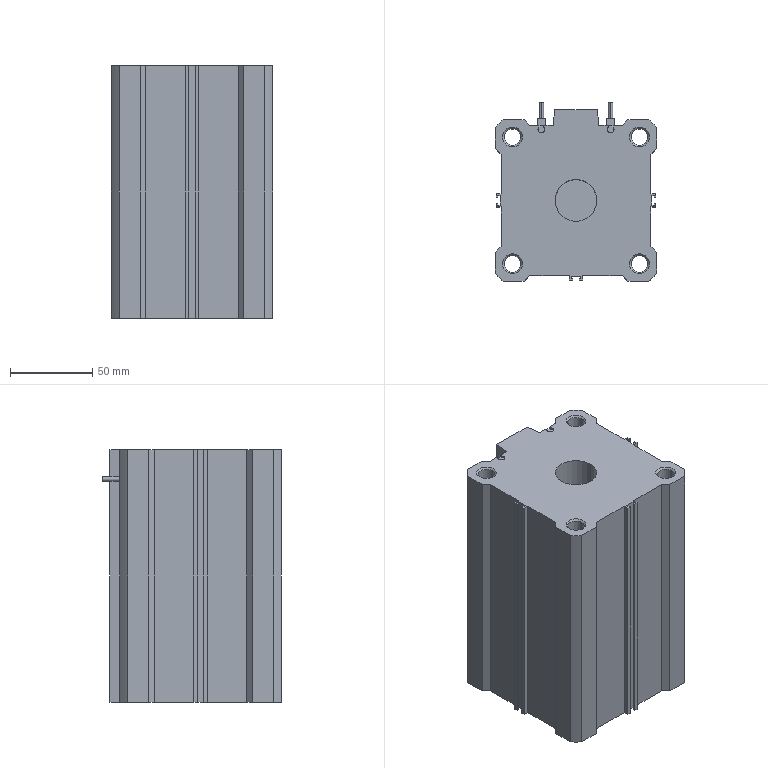Part | STEP file | A_CDQ2A80-100DM-F9NV (Barrel) | 1 solid | 153 faces | box 98 x 108.4 x 153.5 mm | volume 1262277 mm3 | plane 95 | cylinder 34 | cone 20 | spline 4 | commonest cylinder face diameters 10.11 x8 4 x6 4.2 x6 2.7 x4 14.95 x4 132 x4